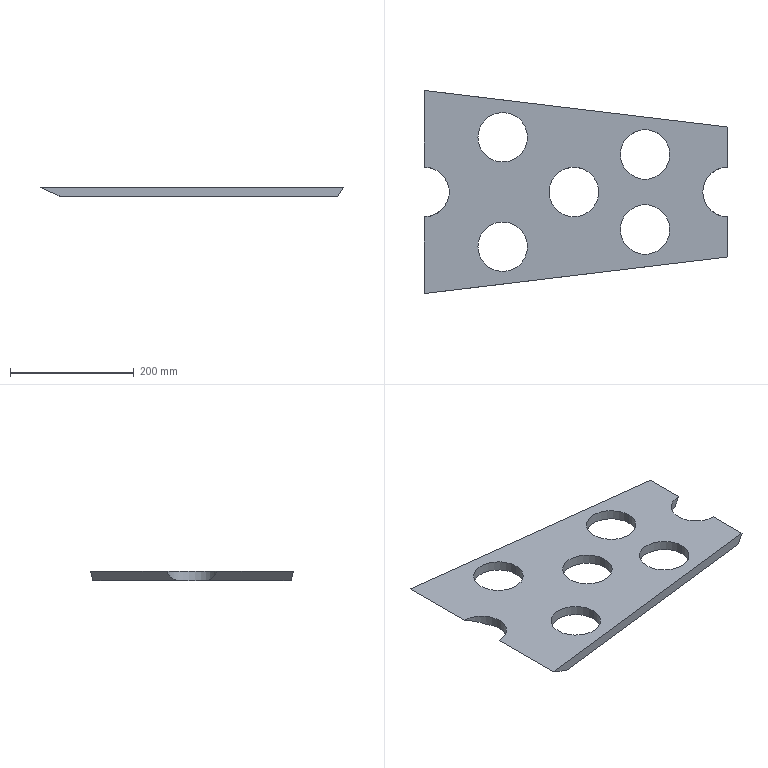Part | SolidWorks | features Extrusion 1, ICE 1 | 1 solid | 21 faces | box 489.6 x 328 x 16 mm | volume 1548186 mm3 | cylinder 13 | plane 8 | commonest cylinder face diameters 80 x13
STEP:
#1=CARTESIAN_POINT('',(316.4,-60.617,16.));
#2=VERTEX_POINT('',#1);
#3=CARTESIAN_POINT('',(396.4,-60.617,16.));
#4=VERTEX_POINT('',#3);
#5=CARTESIAN_POINT('',(356.4,-60.617,16.));
#6=DIRECTION('',(0.,0.,1.));
#7=DIRECTION('',(1.,0.,0.));
#8=AXIS2_PLACEMENT_3D('',#5,#6,#7);
#9=CIRCLE('',#8,40.);
#10=EDGE_CURVE('',#2,#4,#9,.T.);
#11=ORIENTED_EDGE('',*,*,#10,.T.);
#12=CARTESIAN_POINT('',(396.4,-60.617,0.));
#13=VERTEX_POINT('',#12);
#14=CARTESIAN_POINT('',(396.4,-60.617,16.));
#15=DIRECTION('',(0.,0.,-1.));
#16=VECTOR('',#15,1000.);
#17=LINE('',#14,#16);
#18=EDGE_CURVE('',#4,#13,#17,.T.);
#19=ORIENTED_EDGE('',*,*,#18,.T.);
#20=CARTESIAN_POINT('',(316.4,-60.617,0.));
#21=VERTEX_POINT('',#20);
#22=CARTESIAN_POINT('',(356.4,-60.617,0.));
#23=DIRECTION('',(0.,0.,1.));
#24=DIRECTION('',(1.,0.,0.));
#25=AXIS2_PLACEMENT_3D('',#22,#23,#24);
#26=CIRCLE('',#25,40.);
#27=EDGE_CURVE('',#21,#13,#26,.T.);
#28=ORIENTED_EDGE('',*,*,#27,.F.);
#29=CARTESIAN_POINT('',(316.4,-60.617,16.));
#30=DIRECTION('',(0.,0.,-1.));
#31=VECTOR('',#30,1000.);
#32=LINE('',#29,#31);
#33=EDGE_CURVE('',#2,#21,#32,.T.);
#34=ORIENTED_EDGE('',*,*,#33,.F.);
#35=EDGE_LOOP('',(#11,#19,#28,#34));
#36=FACE_OUTER_BOUND('',#35,.T.);
#37=CARTESIAN_POINT('',(356.4,-60.617,16.));
#38=DIRECTION('',(0.,0.,-1.));
#39=DIRECTION('',(-1.,0.,0.));
#40=AXIS2_PLACEMENT_3D('',#37,#38,#39);
#41=CYLINDRICAL_SURFACE('',#40,40.);
#42=ADVANCED_FACE('',(#36),#41,.F.);
#43=CARTESIAN_POINT('',(86.4,-88.334,16.));
#44=VERTEX_POINT('',#43);
#45=CARTESIAN_POINT('',(166.4,-88.334,16.));
#46=VERTEX_POINT('',#45);
#47=CARTESIAN_POINT('',(126.4,-88.334,16.));
#48=DIRECTION('',(0.,0.,1.));
#49=DIRECTION('',(1.,0.,0.));
#50=AXIS2_PLACEMENT_3D('',#47,#48,#49);
#51=CIRCLE('',#50,40.);
#52=EDGE_CURVE('',#44,#46,#51,.T.);
#53=ORIENTED_EDGE('',*,*,#52,.T.);
#54=CARTESIAN_POINT('',(166.4,-88.334,0.));
#55=VERTEX_POINT('',#54);
#56=CARTESIAN_POINT('',(166.4,-88.334,16.));
#57=DIRECTION('',(0.,0.,-1.));
#58=VECTOR('',#57,1000.);
#59=LINE('',#56,#58);
#60=EDGE_CURVE('',#46,#55,#59,.T.);
#61=ORIENTED_EDGE('',*,*,#60,.T.);
#62=CARTESIAN_POINT('',(86.4,-88.334,0.));
#63=VERTEX_POINT('',#62);
#64=CARTESIAN_POINT('',(126.4,-88.334,0.));
#65=DIRECTION('',(0.,0.,1.));
#66=DIRECTION('',(1.,0.,0.));
#67=AXIS2_PLACEMENT_3D('',#64,#65,#66);
#68=CIRCLE('',#67,40.);
#69=EDGE_CURVE('',#63,#55,#68,.T.);
#70=ORIENTED_EDGE('',*,*,#69,.F.);
#71=CARTESIAN_POINT('',(86.4,-88.334,16.));
#72=DIRECTION('',(0.,0.,-1.));
#73=VECTOR('',#72,1000.);
#74=LINE('',#71,#73);
#75=EDGE_CURVE('',#44,#63,#74,.T.);
#76=ORIENTED_EDGE('',*,*,#75,.F.);
#77=EDGE_LOOP('',(#53,#61,#70,#76));
#78=FACE_OUTER_BOUND('',#77,.T.);
#79=CARTESIAN_POINT('',(126.4,-88.334,16.));
#80=DIRECTION('',(0.,0.,-1.));
#81=DIRECTION('',(-1.,0.,0.));
#82=AXIS2_PLACEMENT_3D('',#79,#80,#81);
#83=CYLINDRICAL_SURFACE('',#82,40.);
#84=ADVANCED_FACE('',(#78),#83,.F.);
#85=CARTESIAN_POINT('',(316.4,60.617,16.));
#86=VERTEX_POINT('',#85);
#87=CARTESIAN_POINT('',(396.4,60.617,16.));
#88=VERTEX_POINT('',#87);
#89=CARTESIAN_POINT('',(356.4,60.617,16.));
#90=DIRECTION('',(0.,0.,1.));
#91=DIRECTION('',(1.,0.,0.));
#92=AXIS2_PLACEMENT_3D('',#89,#90,#91);
#93=CIRCLE('',#92,40.);
#94=EDGE_CURVE('',#86,#88,#93,.T.);
#95=ORIENTED_EDGE('',*,*,#94,.T.);
#96=CARTESIAN_POINT('',(396.4,60.617,0.));
#97=VERTEX_POINT('',#96);
#98=CARTESIAN_POINT('',(396.4,60.617,16.));
#99=DIRECTION('',(0.,0.,-1.));
#100=VECTOR('',#99,1000.);
#101=LINE('',#98,#100);
#102=EDGE_CURVE('',#88,#97,#101,.T.);
#103=ORIENTED_EDGE('',*,*,#102,.T.);
#104=CARTESIAN_POINT('',(316.4,60.617,0.));
#105=VERTEX_POINT('',#104);
#106=CARTESIAN_POINT('',(356.4,60.617,0.));
#107=DIRECTION('',(0.,0.,1.));
#108=DIRECTION('',(1.,0.,0.));
#109=AXIS2_PLACEMENT_3D('',#106,#107,#108);
#110=CIRCLE('',#109,40.);
#111=EDGE_CURVE('',#105,#97,#110,.T.);
#112=ORIENTED_EDGE('',*,*,#111,.F.);
#113=CARTESIAN_POINT('',(316.4,60.617,16.));
#114=DIRECTION('',(0.,0.,-1.));
#115=VECTOR('',#114,1000.);
#116=LINE('',#113,#115);
#117=EDGE_CURVE('',#86,#105,#116,.T.);
#118=ORIENTED_EDGE('',*,*,#117,.F.);
#119=EDGE_LOOP('',(#95,#103,#112,#118));
#120=FACE_OUTER_BOUND('',#119,.T.);
#121=CARTESIAN_POINT('',(356.4,60.617,16.));
#122=DIRECTION('',(0.,0.,-1.));
#123=DIRECTION('',(-1.,0.,0.));
#124=AXIS2_PLACEMENT_3D('',#121,#122,#123);
#125=CYLINDRICAL_SURFACE('',#124,40.);
#126=ADVANCED_FACE('',(#120),#125,.F.);
#127=CARTESIAN_POINT('',(86.4,88.334,16.));
#128=VERTEX_POINT('',#127);
#129=CARTESIAN_POINT('',(166.4,88.334,16.));
#130=VERTEX_POINT('',#129);
#131=CARTESIAN_POINT('',(126.4,88.334,16.));
#132=DIRECTION('',(0.,0.,1.));
#133=DIRECTION('',(1.,0.,0.));
#134=AXIS2_PLACEMENT_3D('',#131,#132,#133);
#135=CIRCLE('',#134,40.);
#136=EDGE_CURVE('',#128,#130,#135,.T.);
#137=ORIENTED_EDGE('',*,*,#136,.T.);
#138=CARTESIAN_POINT('',(166.4,88.334,0.));
#139=VERTEX_POINT('',#138);
#140=CARTESIAN_POINT('',(166.4,88.334,16.));
#141=DIRECTION('',(0.,0.,-1.));
#142=VECTOR('',#141,1000.);
#143=LINE('',#140,#142);
#144=EDGE_CURVE('',#130,#139,#143,.T.);
#145=ORIENTED_EDGE('',*,*,#144,.T.);
#146=CARTESIAN_POINT('',(86.4,88.334,0.));
#147=VERTEX_POINT('',#146);
#148=CARTESIAN_POINT('',(126.4,88.334,0.));
#149=DIRECTION('',(0.,0.,1.));
#150=DIRECTION('',(1.,0.,0.));
#151=AXIS2_PLACEMENT_3D('',#148,#149,#150);
#152=CIRCLE('',#151,40.);
#153=EDGE_CURVE('',#147,#139,#152,.T.);
#154=ORIENTED_EDGE('',*,*,#153,.F.);
#155=CARTESIAN_POINT('',(86.4,88.334,16.));
#156=DIRECTION('',(0.,0.,-1.));
#157=VECTOR('',#156,1000.);
#158=LINE('',#155,#157);
#159=EDGE_CURVE('',#128,#147,#158,.T.);
#160=ORIENTED_EDGE('',*,*,#159,.F.);
#161=EDGE_LOOP('',(#137,#145,#154,#160));
#162=FACE_OUTER_BOUND('',#161,.T.);
#163=CARTESIAN_POINT('',(126.4,88.334,16.));
#164=DIRECTION('',(0.,0.,-1.));
#165=DIRECTION('',(-1.,0.,0.));
#166=AXIS2_PLACEMENT_3D('',#163,#164,#165);
#167=CYLINDRICAL_SURFACE('',#166,40.);
#168=ADVANCED_FACE('',(#162),#167,.F.);
#169=CARTESIAN_POINT('',(201.4,0.,16.));
#170=VERTEX_POINT('',#169);
#171=CARTESIAN_POINT('',(281.4,0.,16.));
#172=VERTEX_POINT('',#171);
#173=CARTESIAN_POINT('',(241.4,0.,16.));
#174=DIRECTION('',(0.,0.,1.));
#175=DIRECTION('',(1.,0.,0.));
#176=AXIS2_PLACEMENT_3D('',#173,#174,#175);
#177=CIRCLE('',#176,40.);
#178=EDGE_CURVE('',#170,#172,#177,.T.);
#179=ORIENTED_EDGE('',*,*,#178,.T.);
#180=CARTESIAN_POINT('',(281.4,0.,0.));
#181=VERTEX_POINT('',#180);
#182=CARTESIAN_POINT('',(281.4,0.,16.));
#183=DIRECTION('',(0.,0.,-1.));
#184=VECTOR('',#183,1000.);
#185=LINE('',#182,#184);
#186=EDGE_CURVE('',#172,#181,#185,.T.);
#187=ORIENTED_EDGE('',*,*,#186,.T.);
#188=CARTESIAN_POINT('',(201.4,0.,0.));
#189=VERTEX_POINT('',#188);
#190=CARTESIAN_POINT('',(241.4,0.,0.));
#191=DIRECTION('',(0.,0.,1.));
#192=DIRECTION('',(1.,0.,0.));
#193=AXIS2_PLACEMENT_3D('',#190,#191,#192);
#194=CIRCLE('',#193,40.);
#195=EDGE_CURVE('',#189,#181,#194,.T.);
#196=ORIENTED_EDGE('',*,*,#195,.F.);
#197=CARTESIAN_POINT('',(201.4,0.,16.));
#198=DIRECTION('',(0.,0.,-1.));
#199=VECTOR('',#198,1000.);
#200=LINE('',#197,#199);
#201=EDGE_CURVE('',#170,#189,#200,.T.);
#202=ORIENTED_EDGE('',*,*,#201,.F.);
#203=EDGE_LOOP('',(#179,#187,#196,#202));
#204=FACE_OUTER_BOUND('',#203,.T.);
#205=CARTESIAN_POINT('',(241.4,0.,16.));
#206=DIRECTION('',(0.,0.,-1.));
#207=DIRECTION('',(-1.,0.,0.));
#208=AXIS2_PLACEMENT_3D('',#205,#206,#207);
#209=CYLINDRICAL_SURFACE('',#208,40.);
#210=ADVANCED_FACE('',(#204),#209,.F.);
#211=CARTESIAN_POINT('',(449.6,0.,16.));
#212=VERTEX_POINT('',#211);
#213=CARTESIAN_POINT('',(489.6,40.,16.));
#214=VERTEX_POINT('',#213);
#215=CARTESIAN_POINT('',(489.6,0.,16.));
#216=DIRECTION('',(0.,0.,-1.));
#217=DIRECTION('',(1.,0.,0.));
#218=AXIS2_PLACEMENT_3D('',#215,#216,#217);
#219=CIRCLE('',#218,40.);
#220=EDGE_CURVE('',#212,#214,#219,.T.);
#221=ORIENTED_EDGE('',*,*,#220,.F.);
#222=CARTESIAN_POINT('',(449.6,0.,0.));
#223=VERTEX_POINT('',#222);
#224=CARTESIAN_POINT('',(449.6,0.,16.));
#225=DIRECTION('',(0.,0.,-1.));
#226=VECTOR('',#225,1000.);
#227=LINE('',#224,#226);
#228=EDGE_CURVE('',#212,#223,#227,.T.);
#229=ORIENTED_EDGE('',*,*,#228,.T.);
#230=CARTESIAN_POINT('',(480.168,38.872,0.));
#231=VERTEX_POINT('',#230);
#232=CARTESIAN_POINT('',(489.6,0.,0.));
#233=DIRECTION('',(0.,0.,-1.));
#234=DIRECTION('',(1.,0.,0.));
#235=AXIS2_PLACEMENT_3D('',#232,#233,#234);
#236=CIRCLE('',#235,40.);
#237=EDGE_CURVE('',#223,#231,#236,.T.);
#238=ORIENTED_EDGE('',*,*,#237,.T.);
#239=CARTESIAN_POINT('',(480.168,38.872,0.));
#240=CARTESIAN_POINT('',(483.26,39.622,5.245));
#241=CARTESIAN_POINT('',(486.419,40.,10.603));
#242=CARTESIAN_POINT('',(489.6,40.,16.));
#243=(BOUNDED_CURVE()B_SPLINE_CURVE(3,(#239,#240,#241,#242),.UNSPECIFIED.,.F.,.F.)B_SPLINE_CURVE_WITH_KNOTS((4,4),(1.333,1.571),.UNSPECIFIED.)CURVE()GEOMETRIC_REPRESENTATION_ITEM()RATIONAL_B_SPLINE_CURVE((1.,0.9953,0.9953,1.))REPRESENTATION_ITEM(''));
#244=EDGE_CURVE('',#231,#214,#243,.T.);
#245=ORIENTED_EDGE('',*,*,#244,.T.);
#246=EDGE_LOOP('',(#221,#229,#238,#245));
#247=FACE_OUTER_BOUND('',#246,.T.);
#248=CARTESIAN_POINT('',(489.6,0.,16.));
#249=DIRECTION('',(0.,0.,-1.));
#250=DIRECTION('',(-1.,0.,0.));
#251=AXIS2_PLACEMENT_3D('',#248,#249,#250);
#252=CYLINDRICAL_SURFACE('',#251,40.);
#253=ADVANCED_FACE('',(#247),#252,.F.);
#254=ORIENTED_EDGE('',*,*,#52,.F.);
#255=CARTESIAN_POINT('',(126.4,-88.334,16.));
#256=DIRECTION('',(0.,0.,1.));
#257=DIRECTION('',(1.,0.,0.));
#258=AXIS2_PLACEMENT_3D('',#255,#256,#257);
#259=CIRCLE('',#258,40.);
#260=EDGE_CURVE('',#46,#44,#259,.T.);
#261=ORIENTED_EDGE('',*,*,#260,.F.);
#262=EDGE_LOOP('',(#254,#261));
#263=FACE_BOUND('',#262,.T.);
#264=ORIENTED_EDGE('',*,*,#136,.F.);
#265=CARTESIAN_POINT('',(126.4,88.334,16.));
#266=DIRECTION('',(0.,0.,1.));
#267=DIRECTION('',(1.,0.,0.));
#268=AXIS2_PLACEMENT_3D('',#265,#266,#267);
#269=CIRCLE('',#268,40.);
#270=EDGE_CURVE('',#130,#128,#269,.T.);
#271=ORIENTED_EDGE('',*,*,#270,.F.);
#272=EDGE_LOOP('',(#264,#271));
#273=FACE_BOUND('',#272,.T.);
#274=CARTESIAN_POINT('',(489.6,105.,16.));
#275=VERTEX_POINT('',#274);
#276=CARTESIAN_POINT('',(0.,164.,16.));
#277=VERTEX_POINT('',#276);
#278=CARTESIAN_POINT('',(0.,164.,16.));
#279=DIRECTION('',(-0.9928,0.1196,0.));
#280=VECTOR('',#279,1000.);
#281=LINE('',#278,#280);
#282=EDGE_CURVE('',#275,#277,#281,.T.);
#283=ORIENTED_EDGE('',*,*,#282,.T.);
#284=CARTESIAN_POINT('',(0.,40.,16.));
#285=VERTEX_POINT('',#284);
#286=CARTESIAN_POINT('',(0.,40.,16.));
#287=DIRECTION('',(0.,-1.,0.));
#288=VECTOR('',#287,1000.);
#289=LINE('',#286,#288);
#290=EDGE_CURVE('',#277,#285,#289,.T.);
#291=ORIENTED_EDGE('',*,*,#290,.T.);
#292=CARTESIAN_POINT('',(0.,-40.,16.));
#293=VERTEX_POINT('',#292);
#294=CARTESIAN_POINT('',(0.,0.,16.));
#295=DIRECTION('',(0.,0.,-1.));
#296=DIRECTION('',(1.,0.,0.));
#297=AXIS2_PLACEMENT_3D('',#294,#295,#296);
#298=CIRCLE('',#297,40.);
#299=EDGE_CURVE('',#285,#293,#298,.T.);
#300=ORIENTED_EDGE('',*,*,#299,.T.);
#301=CARTESIAN_POINT('',(0.,-164.,16.));
#302=VERTEX_POINT('',#301);
#303=CARTESIAN_POINT('',(0.,-40.,16.));
#304=DIRECTION('',(0.,-1.,0.));
#305=VECTOR('',#304,1000.);
#306=LINE('',#303,#305);
#307=EDGE_CURVE('',#293,#302,#306,.T.);
#308=ORIENTED_EDGE('',*,*,#307,.T.);
#309=CARTESIAN_POINT('',(489.6,-105.,16.));
#310=VERTEX_POINT('',#309);
#311=CARTESIAN_POINT('',(0.,-164.,16.));
#312=DIRECTION('',(0.9928,0.1196,0.));
#313=VECTOR('',#312,1000.);
#314=LINE('',#311,#313);
#315=EDGE_CURVE('',#302,#310,#314,.T.);
#316=ORIENTED_EDGE('',*,*,#315,.T.);
#317=CARTESIAN_POINT('',(489.6,-40.,16.));
#318=VERTEX_POINT('',#317);
#319=CARTESIAN_POINT('',(489.6,-105.,16.));
#320=DIRECTION('',(0.,1.,0.));
#321=VECTOR('',#320,1000.);
#322=LINE('',#319,#321);
#323=EDGE_CURVE('',#310,#318,#322,.T.);
#324=ORIENTED_EDGE('',*,*,#323,.T.);
#325=CARTESIAN_POINT('',(489.6,0.,16.));
#326=DIRECTION('',(0.,0.,-1.));
#327=DIRECTION('',(1.,0.,0.));
#328=AXIS2_PLACEMENT_3D('',#325,#326,#327);
#329=CIRCLE('',#328,40.);
#330=EDGE_CURVE('',#318,#212,#329,.T.);
#331=ORIENTED_EDGE('',*,*,#330,.T.);
#332=ORIENTED_EDGE('',*,*,#220,.T.);
#333=CARTESIAN_POINT('',(489.6,105.,16.));
#334=DIRECTION('',(0.,1.,0.));
#335=VECTOR('',#334,1000.);
#336=LINE('',#333,#335);
#337=EDGE_CURVE('',#214,#275,#336,.T.);
#338=ORIENTED_EDGE('',*,*,#337,.T.);
#339=EDGE_LOOP('',(#283,#291,#300,#308,#316,#324,#331,#332,#338));
#340=FACE_OUTER_BOUND('',#339,.T.);
#341=ORIENTED_EDGE('',*,*,#178,.F.);
#342=CARTESIAN_POINT('',(241.4,0.,16.));
#343=DIRECTION('',(0.,0.,1.));
#344=DIRECTION('',(1.,0.,0.));
#345=AXIS2_PLACEMENT_3D('',#342,#343,#344);
#346=CIRCLE('',#345,40.);
#347=EDGE_CURVE('',#172,#170,#346,.T.);
#348=ORIENTED_EDGE('',*,*,#347,.F.);
#349=EDGE_LOOP('',(#341,#348));
#350=FACE_BOUND('',#349,.T.);
#351=ORIENTED_EDGE('',*,*,#94,.F.);
#352=CARTESIAN_POINT('',(356.4,60.617,16.));
#353=DIRECTION('',(0.,0.,1.));
#354=DIRECTION('',(1.,0.,0.));
#355=AXIS2_PLACEMENT_3D('',#352,#353,#354);
#356=CIRCLE('',#355,40.);
#357=EDGE_CURVE('',#88,#86,#356,.T.);
#358=ORIENTED_EDGE('',*,*,#357,.F.);
#359=EDGE_LOOP('',(#351,#358));
#360=FACE_BOUND('',#359,.T.);
#361=ORIENTED_EDGE('',*,*,#10,.F.);
#362=CARTESIAN_POINT('',(356.4,-60.617,16.));
#363=DIRECTION('',(0.,0.,1.));
#364=DIRECTION('',(1.,0.,0.));
#365=AXIS2_PLACEMENT_3D('',#362,#363,#364);
#366=CIRCLE('',#365,40.);
#367=EDGE_CURVE('',#4,#2,#366,.T.);
#368=ORIENTED_EDGE('',*,*,#367,.F.);
#369=EDGE_LOOP('',(#361,#368));
#370=FACE_BOUND('',#369,.T.);
#371=CARTESIAN_POINT('',(489.6,0.,16.));
#372=DIRECTION('',(0.,0.,1.));
#373=DIRECTION('',(1.,0.,0.));
#374=AXIS2_PLACEMENT_3D('',#371,#372,#373);
#375=PLANE('',#374);
#376=ADVANCED_FACE('',(#263,#273,#340,#350,#360,#370),#375,.T.);
#377=ORIENTED_EDGE('',*,*,#69,.T.);
#378=CARTESIAN_POINT('',(126.4,-88.334,0.));
#379=DIRECTION('',(0.,0.,1.));
#380=DIRECTION('',(1.,0.,0.));
#381=AXIS2_PLACEMENT_3D('',#378,#379,#380);
#382=CIRCLE('',#381,40.);
#383=EDGE_CURVE('',#55,#63,#382,.T.);
#384=ORIENTED_EDGE('',*,*,#383,.T.);
#385=EDGE_LOOP('',(#377,#384));
#386=FACE_BOUND('',#385,.T.);
#387=ORIENTED_EDGE('',*,*,#153,.T.);
#388=CARTESIAN_POINT('',(126.4,88.334,0.));
#389=DIRECTION('',(0.,0.,1.));
#390=DIRECTION('',(1.,0.,0.));
#391=AXIS2_PLACEMENT_3D('',#388,#389,#390);
#392=CIRCLE('',#391,40.);
#393=EDGE_CURVE('',#139,#147,#392,.T.);
#394=ORIENTED_EDGE('',*,*,#393,.T.);
#395=EDGE_LOOP('',(#387,#394));
#396=FACE_BOUND('',#395,.T.);
#397=CARTESIAN_POINT('',(33.259,-159.992,0.));
#398=VERTEX_POINT('',#397);
#399=CARTESIAN_POINT('',(480.168,-106.137,0.));
#400=VERTEX_POINT('',#399);
#401=CARTESIAN_POINT('',(0.,-164.,0.));
#402=DIRECTION('',(0.9928,0.1196,0.));
#403=VECTOR('',#402,1000.);
#404=LINE('',#401,#403);
#405=EDGE_CURVE('',#398,#400,#404,.T.);
#406=ORIENTED_EDGE('',*,*,#405,.F.);
#407=CARTESIAN_POINT('',(33.259,-22.222,0.));
#408=VERTEX_POINT('',#407);
#409=CARTESIAN_POINT('',(33.259,340.008,0.));
#410=DIRECTION('',(0.,-1.,0.));
#411=VECTOR('',#410,1000.);
#412=LINE('',#409,#411);
#413=EDGE_CURVE('',#408,#398,#412,.T.);
#414=ORIENTED_EDGE('',*,*,#413,.F.);
#415=CARTESIAN_POINT('',(33.259,22.222,0.));
#416=VERTEX_POINT('',#415);
#417=CARTESIAN_POINT('',(0.,0.,0.));
#418=DIRECTION('',(0.,0.,-1.));
#419=DIRECTION('',(1.,0.,0.));
#420=AXIS2_PLACEMENT_3D('',#417,#418,#419);
#421=CIRCLE('',#420,40.);
#422=EDGE_CURVE('',#416,#408,#421,.T.);
#423=ORIENTED_EDGE('',*,*,#422,.F.);
#424=CARTESIAN_POINT('',(33.259,159.992,0.));
#425=VERTEX_POINT('',#424);
#426=CARTESIAN_POINT('',(33.259,340.008,0.));
#427=DIRECTION('',(0.,-1.,0.));
#428=VECTOR('',#427,1000.);
#429=LINE('',#426,#428);
#430=EDGE_CURVE('',#425,#416,#429,.T.);
#431=ORIENTED_EDGE('',*,*,#430,.F.);
#432=CARTESIAN_POINT('',(480.168,106.137,0.));
#433=VERTEX_POINT('',#432);
#434=CARTESIAN_POINT('',(0.,164.,0.));
#435=DIRECTION('',(-0.9928,0.1196,0.));
#436=VECTOR('',#435,1000.);
#437=LINE('',#434,#436);
#438=EDGE_CURVE('',#433,#425,#437,.T.);
#439=ORIENTED_EDGE('',*,*,#438,.F.);
#440=CARTESIAN_POINT('',(480.168,393.863,0.));
#441=DIRECTION('',(0.,-1.,0.));
#442=VECTOR('',#441,1000.);
#443=LINE('',#440,#442);
#444=EDGE_CURVE('',#433,#231,#443,.T.);
#445=ORIENTED_EDGE('',*,*,#444,.T.);
#446=ORIENTED_EDGE('',*,*,#237,.F.);
#447=CARTESIAN_POINT('',(480.168,-38.872,0.));
#448=VERTEX_POINT('',#447);
#449=CARTESIAN_POINT('',(489.6,0.,0.));
#450=DIRECTION('',(0.,0.,-1.));
#451=DIRECTION('',(1.,0.,0.));
#452=AXIS2_PLACEMENT_3D('',#449,#450,#451);
#453=CIRCLE('',#452,40.);
#454=EDGE_CURVE('',#448,#223,#453,.T.);
#455=ORIENTED_EDGE('',*,*,#454,.F.);
#456=CARTESIAN_POINT('',(480.168,393.863,0.));
#457=DIRECTION('',(0.,-1.,0.));
#458=VECTOR('',#457,1000.);
#459=LINE('',#456,#458);
#460=EDGE_CURVE('',#448,#400,#459,.T.);
#461=ORIENTED_EDGE('',*,*,#460,.T.);
#462=EDGE_LOOP('',(#406,#414,#423,#431,#439,#445,#446,#455,#461));
#463=FACE_OUTER_BOUND('',#462,.T.);
#464=ORIENTED_EDGE('',*,*,#195,.T.);
#465=CARTESIAN_POINT('',(241.4,0.,0.));
#466=DIRECTION('',(0.,0.,1.));
#467=DIRECTION('',(1.,0.,0.));
#468=AXIS2_PLACEMENT_3D('',#465,#466,#467);
#469=CIRCLE('',#468,40.);
#470=EDGE_CURVE('',#181,#189,#469,.T.);
#471=ORIENTED_EDGE('',*,*,#470,.T.);
#472=EDGE_LOOP('',(#464,#471));
#473=FACE_BOUND('',#472,.T.);
#474=ORIENTED_EDGE('',*,*,#111,.T.);
#475=CARTESIAN_POINT('',(356.4,60.617,0.));
#476=DIRECTION('',(0.,0.,1.));
#477=DIRECTION('',(1.,0.,0.));
#478=AXIS2_PLACEMENT_3D('',#475,#476,#477);
#479=CIRCLE('',#478,40.);
#480=EDGE_CURVE('',#97,#105,#479,.T.);
#481=ORIENTED_EDGE('',*,*,#480,.T.);
#482=EDGE_LOOP('',(#474,#481));
#483=FACE_BOUND('',#482,.T.);
#484=ORIENTED_EDGE('',*,*,#27,.T.);
#485=CARTESIAN_POINT('',(356.4,-60.617,0.));
#486=DIRECTION('',(0.,0.,1.));
#487=DIRECTION('',(1.,0.,0.));
#488=AXIS2_PLACEMENT_3D('',#485,#486,#487);
#489=CIRCLE('',#488,40.);
#490=EDGE_CURVE('',#13,#21,#489,.T.);
#491=ORIENTED_EDGE('',*,*,#490,.T.);
#492=EDGE_LOOP('',(#484,#491));
#493=FACE_BOUND('',#492,.T.);
#494=CARTESIAN_POINT('',(489.6,0.,0.));
#495=DIRECTION('',(0.,0.,1.));
#496=DIRECTION('',(1.,0.,0.));
#497=AXIS2_PLACEMENT_3D('',#494,#495,#496);
#498=PLANE('',#497);
#499=ADVANCED_FACE('',(#386,#396,#463,#473,#483,#493),#498,.F.);
#500=ORIENTED_EDGE('',*,*,#438,.T.);
#501=CARTESIAN_POINT('',(0.,164.,16.));
#502=DIRECTION('',(-0.8959,0.108,0.431));
#503=VECTOR('',#502,1000.);
#504=LINE('',#501,#503);
#505=EDGE_CURVE('',#425,#277,#504,.T.);
#506=ORIENTED_EDGE('',*,*,#505,.T.);
#507=ORIENTED_EDGE('',*,*,#282,.F.);
#508=CARTESIAN_POINT('',(361.986,120.378,-200.484));
#509=DIRECTION('',(-0.5069,0.06108,-0.8599));
#510=VECTOR('',#509,1000.);
#511=LINE('',#508,#510);
#512=EDGE_CURVE('',#275,#433,#511,.T.);
#513=ORIENTED_EDGE('',*,*,#512,.T.);
#514=EDGE_LOOP('',(#500,#506,#507,#513));
#515=FACE_OUTER_BOUND('',#514,.T.);
#516=CARTESIAN_POINT('',(0.,164.,16.));
#517=DIRECTION('',(-0.1196,-0.9928,0.));
#518=DIRECTION('',(0.9928,-0.1196,0.));
#519=AXIS2_PLACEMENT_3D('',#516,#517,#518);
#520=PLANE('',#519);
#521=ADVANCED_FACE('',(#515),#520,.F.);
#522=ORIENTED_EDGE('',*,*,#422,.T.);
#523=CARTESIAN_POINT('',(33.259,-22.222,0.));
#524=CARTESIAN_POINT('',(25.679,-33.568,3.647));
#525=CARTESIAN_POINT('',(13.645,-40.,9.436));
#526=CARTESIAN_POINT('',(0.,-40.,16.));
#527=(BOUNDED_CURVE()B_SPLINE_CURVE(3,(#523,#524,#525,#526),.UNSPECIFIED.,.F.,.F.)B_SPLINE_CURVE_WITH_KNOTS((4,4),(0.589,1.571),.UNSPECIFIED.)CURVE()GEOMETRIC_REPRESENTATION_ITEM()RATIONAL_B_SPLINE_CURVE((1.,0.9213,0.9213,1.))REPRESENTATION_ITEM(''));
#528=EDGE_CURVE('',#408,#293,#527,.T.);
#529=ORIENTED_EDGE('',*,*,#528,.T.);
#530=ORIENTED_EDGE('',*,*,#299,.F.);
#531=CARTESIAN_POINT('',(0.,40.,16.));
#532=CARTESIAN_POINT('',(13.645,40.,9.436));
#533=CARTESIAN_POINT('',(25.679,33.568,3.647));
#534=CARTESIAN_POINT('',(33.259,22.222,0.));
#535=(BOUNDED_CURVE()B_SPLINE_CURVE(3,(#531,#532,#533,#534),.UNSPECIFIED.,.F.,.F.)B_SPLINE_CURVE_WITH_KNOTS((4,4),(4.712,5.694),.UNSPECIFIED.)CURVE()GEOMETRIC_REPRESENTATION_ITEM()RATIONAL_B_SPLINE_CURVE((1.,0.9213,0.9213,1.))REPRESENTATION_ITEM(''));
#536=EDGE_CURVE('',#285,#416,#535,.T.);
#537=ORIENTED_EDGE('',*,*,#536,.T.);
#538=EDGE_LOOP('',(#522,#529,#530,#537));
#539=FACE_OUTER_BOUND('',#538,.T.);
#540=CARTESIAN_POINT('',(0.,0.,16.));
#541=DIRECTION('',(0.,0.,-1.));
#542=DIRECTION('',(-1.,0.,0.));
#543=AXIS2_PLACEMENT_3D('',#540,#541,#542);
#544=CYLINDRICAL_SURFACE('',#543,40.);
#545=ADVANCED_FACE('',(#539),#544,.F.);
#546=ORIENTED_EDGE('',*,*,#315,.F.);
#547=CARTESIAN_POINT('',(0.,-164.,16.));
#548=DIRECTION('',(-0.8959,-0.108,0.431));
#549=VECTOR('',#548,1000.);
#550=LINE('',#547,#549);
#551=EDGE_CURVE('',#398,#302,#550,.T.);
#552=ORIENTED_EDGE('',*,*,#551,.F.);
#553=ORIENTED_EDGE('',*,*,#405,.T.);
#554=CARTESIAN_POINT('',(489.6,-105.,16.));
#555=DIRECTION('',(-0.5069,-0.06108,-0.8599));
#556=VECTOR('',#555,1000.);
#557=LINE('',#554,#556);
#558=EDGE_CURVE('',#310,#400,#557,.T.);
#559=ORIENTED_EDGE('',*,*,#558,.F.);
#560=EDGE_LOOP('',(#546,#552,#553,#559));
#561=FACE_OUTER_BOUND('',#560,.T.);
#562=CARTESIAN_POINT('',(0.,-164.,16.));
#563=DIRECTION('',(-0.1196,0.9928,0.));
#564=DIRECTION('',(-0.9928,-0.1196,0.));
#565=AXIS2_PLACEMENT_3D('',#562,#563,#564);
#566=PLANE('',#565);
#567=ADVANCED_FACE('',(#561),#566,.F.);
#568=ORIENTED_EDGE('',*,*,#228,.F.);
#569=ORIENTED_EDGE('',*,*,#330,.F.);
#570=CARTESIAN_POINT('',(489.6,-40.,16.));
#571=CARTESIAN_POINT('',(486.419,-40.,10.603));
#572=CARTESIAN_POINT('',(483.26,-39.622,5.245));
#573=CARTESIAN_POINT('',(480.168,-38.872,0.));
#574=(BOUNDED_CURVE()B_SPLINE_CURVE(3,(#570,#571,#572,#573),.UNSPECIFIED.,.F.,.F.)B_SPLINE_CURVE_WITH_KNOTS((4,4),(4.712,4.95),.UNSPECIFIED.)CURVE()GEOMETRIC_REPRESENTATION_ITEM()RATIONAL_B_SPLINE_CURVE((1.,0.9953,0.9953,1.))REPRESENTATION_ITEM(''));
#575=EDGE_CURVE('',#318,#448,#574,.T.);
#576=ORIENTED_EDGE('',*,*,#575,.T.);
#577=ORIENTED_EDGE('',*,*,#454,.T.);
#578=EDGE_LOOP('',(#568,#569,#576,#577));
#579=FACE_OUTER_BOUND('',#578,.T.);
#580=CARTESIAN_POINT('',(489.6,0.,16.));
#581=DIRECTION('',(0.,0.,-1.));
#582=DIRECTION('',(-1.,0.,0.));
#583=AXIS2_PLACEMENT_3D('',#580,#581,#582);
#584=CYLINDRICAL_SURFACE('',#583,40.);
#585=ADVANCED_FACE('',(#579),#584,.F.);
#586=ORIENTED_EDGE('',*,*,#186,.F.);
#587=ORIENTED_EDGE('',*,*,#347,.T.);
#588=ORIENTED_EDGE('',*,*,#201,.T.);
#589=ORIENTED_EDGE('',*,*,#470,.F.);
#590=EDGE_LOOP('',(#586,#587,#588,#589));
#591=FACE_OUTER_BOUND('',#590,.T.);
#592=CARTESIAN_POINT('',(241.4,0.,16.));
#593=DIRECTION('',(0.,0.,-1.));
#594=DIRECTION('',(-1.,0.,0.));
#595=AXIS2_PLACEMENT_3D('',#592,#593,#594);
#596=CYLINDRICAL_SURFACE('',#595,40.);
#597=ADVANCED_FACE('',(#591),#596,.F.);
#598=ORIENTED_EDGE('',*,*,#144,.F.);
#599=ORIENTED_EDGE('',*,*,#270,.T.);
#600=ORIENTED_EDGE('',*,*,#159,.T.);
#601=ORIENTED_EDGE('',*,*,#393,.F.);
#602=EDGE_LOOP('',(#598,#599,#600,#601));
#603=FACE_OUTER_BOUND('',#602,.T.);
#604=CARTESIAN_POINT('',(126.4,88.334,16.));
#605=DIRECTION('',(0.,0.,-1.));
#606=DIRECTION('',(-1.,0.,0.));
#607=AXIS2_PLACEMENT_3D('',#604,#605,#606);
#608=CYLINDRICAL_SURFACE('',#607,40.);
#609=ADVANCED_FACE('',(#603),#608,.F.);
#610=ORIENTED_EDGE('',*,*,#102,.F.);
#611=ORIENTED_EDGE('',*,*,#357,.T.);
#612=ORIENTED_EDGE('',*,*,#117,.T.);
#613=ORIENTED_EDGE('',*,*,#480,.F.);
#614=EDGE_LOOP('',(#610,#611,#612,#613));
#615=FACE_OUTER_BOUND('',#614,.T.);
#616=CARTESIAN_POINT('',(356.4,60.617,16.));
#617=DIRECTION('',(0.,0.,-1.));
#618=DIRECTION('',(-1.,0.,0.));
#619=AXIS2_PLACEMENT_3D('',#616,#617,#618);
#620=CYLINDRICAL_SURFACE('',#619,40.);
#621=ADVANCED_FACE('',(#615),#620,.F.);
#622=ORIENTED_EDGE('',*,*,#60,.F.);
#623=ORIENTED_EDGE('',*,*,#260,.T.);
#624=ORIENTED_EDGE('',*,*,#75,.T.);
#625=ORIENTED_EDGE('',*,*,#383,.F.);
#626=EDGE_LOOP('',(#622,#623,#624,#625));
#627=FACE_OUTER_BOUND('',#626,.T.);
#628=CARTESIAN_POINT('',(126.4,-88.334,16.));
#629=DIRECTION('',(0.,0.,-1.));
#630=DIRECTION('',(-1.,0.,0.));
#631=AXIS2_PLACEMENT_3D('',#628,#629,#630);
#632=CYLINDRICAL_SURFACE('',#631,40.);
#633=ADVANCED_FACE('',(#627),#632,.F.);
#634=ORIENTED_EDGE('',*,*,#18,.F.);
#635=ORIENTED_EDGE('',*,*,#367,.T.);
#636=ORIENTED_EDGE('',*,*,#33,.T.);
#637=ORIENTED_EDGE('',*,*,#490,.F.);
#638=EDGE_LOOP('',(#634,#635,#636,#637));
#639=FACE_OUTER_BOUND('',#638,.T.);
#640=CARTESIAN_POINT('',(356.4,-60.617,16.));
#641=DIRECTION('',(0.,0.,-1.));
#642=DIRECTION('',(-1.,0.,0.));
#643=AXIS2_PLACEMENT_3D('',#640,#641,#642);
#644=CYLINDRICAL_SURFACE('',#643,40.);
#645=ADVANCED_FACE('',(#639),#644,.F.);
#646=ORIENTED_EDGE('',*,*,#337,.F.);
#647=ORIENTED_EDGE('',*,*,#244,.F.);
#648=ORIENTED_EDGE('',*,*,#444,.F.);
#649=ORIENTED_EDGE('',*,*,#512,.F.);
#650=EDGE_LOOP('',(#646,#647,#648,#649));
#651=FACE_OUTER_BOUND('',#650,.T.);
#652=CARTESIAN_POINT('',(489.6,395.,16.));
#653=DIRECTION('',(-0.8615,0.,0.5078));
#654=DIRECTION('',(0.5078,0.,0.8615));
#655=AXIS2_PLACEMENT_3D('',#652,#653,#654);
#656=PLANE('',#655);
#657=ADVANCED_FACE('',(#651),#656,.F.);
#658=ORIENTED_EDGE('',*,*,#323,.F.);
#659=ORIENTED_EDGE('',*,*,#558,.T.);
#660=ORIENTED_EDGE('',*,*,#460,.F.);
#661=ORIENTED_EDGE('',*,*,#575,.F.);
#662=EDGE_LOOP('',(#658,#659,#660,#661));
#663=FACE_OUTER_BOUND('',#662,.T.);
#664=CARTESIAN_POINT('',(489.6,395.,16.));
#665=DIRECTION('',(-0.8615,0.,0.5078));
#666=DIRECTION('',(0.5078,0.,0.8615));
#667=AXIS2_PLACEMENT_3D('',#664,#665,#666);
#668=PLANE('',#667);
#669=ADVANCED_FACE('',(#663),#668,.F.);
#670=ORIENTED_EDGE('',*,*,#413,.T.);
#671=ORIENTED_EDGE('',*,*,#551,.T.);
#672=ORIENTED_EDGE('',*,*,#307,.F.);
#673=ORIENTED_EDGE('',*,*,#528,.F.);
#674=EDGE_LOOP('',(#670,#671,#672,#673));
#675=FACE_OUTER_BOUND('',#674,.T.);
#676=CARTESIAN_POINT('',(0.,336.,16.));
#677=DIRECTION('',(0.4335,0.,0.9011));
#678=DIRECTION('',(0.9011,0.,-0.4335));
#679=AXIS2_PLACEMENT_3D('',#676,#677,#678);
#680=PLANE('',#679);
#681=ADVANCED_FACE('',(#675),#680,.F.);
#682=ORIENTED_EDGE('',*,*,#430,.T.);
#683=ORIENTED_EDGE('',*,*,#536,.F.);
#684=ORIENTED_EDGE('',*,*,#290,.F.);
#685=ORIENTED_EDGE('',*,*,#505,.F.);
#686=EDGE_LOOP('',(#682,#683,#684,#685));
#687=FACE_OUTER_BOUND('',#686,.T.);
#688=CARTESIAN_POINT('',(0.,336.,16.));
#689=DIRECTION('',(0.4335,0.,0.9011));
#690=DIRECTION('',(0.9011,0.,-0.4335));
#691=AXIS2_PLACEMENT_3D('',#688,#689,#690);
#692=PLANE('',#691);
#693=ADVANCED_FACE('',(#687),#692,.F.);
#694=CLOSED_SHELL('',(#42,#84,#126,#168,#210,#253,#376,#499,#521,#545,#567,#585,#597,#609,#621,#633,#645,#657,#669,#681,#693));
#695=MANIFOLD_SOLID_BREP('',#694);
#696=CARTESIAN_POINT('',(0.,0.,0.));
#697=DIRECTION('',(0.,0.,1.));
#698=DIRECTION('',(1.,0.,0.));
#699=AXIS2_PLACEMENT_3D('',#696,#697,#698);
#700=(LENGTH_UNIT()NAMED_UNIT(*)SI_UNIT(.MILLI.,.METRE.));
#701=UNCERTAINTY_MEASURE_WITH_UNIT(LENGTH_MEASURE(0.00001),#700,'','');
#702=(NAMED_UNIT(*)PLANE_ANGLE_UNIT()SI_UNIT($,.RADIAN.));
#703=(NAMED_UNIT(*)SI_UNIT($,.STERADIAN.)SOLID_ANGLE_UNIT());
#704=(GEOMETRIC_REPRESENTATION_CONTEXT(3)GLOBAL_UNCERTAINTY_ASSIGNED_CONTEXT((#701))GLOBAL_UNIT_ASSIGNED_CONTEXT((#700,#702,#703))REPRESENTATION_CONTEXT('',''));
#705=ADVANCED_BREP_SHAPE_REPRESENTATION('',(#695,#699),#704);